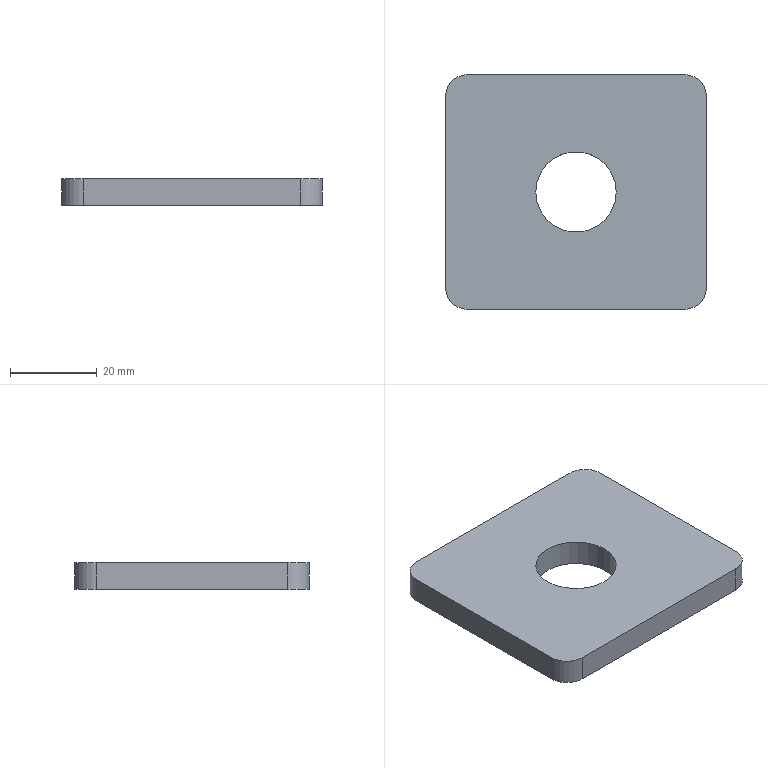Part | STEP file | JBJ-P-1015-03 | 1 solid | 11 faces | box 60 x 54 x 6 mm | volume 17698 mm3 | plane 6 | cylinder 5 | commonest cylinder face diameters 10 x4 18.5 x1
STEP:
#1=CARTESIAN_POINT('',(0.,-5.,0.));
#2=VERTEX_POINT('',#1);
#3=CARTESIAN_POINT('',(0.,-49.,0.));
#4=VERTEX_POINT('',#3);
#5=CARTESIAN_POINT('',(0.,0.,0.));
#6=DIRECTION('',(0.,-1.,0.));
#7=VECTOR('',#6,1000.);
#8=LINE('',#5,#7);
#9=EDGE_CURVE('',#2,#4,#8,.T.);
#10=ORIENTED_EDGE('',*,*,#9,.T.);
#11=CARTESIAN_POINT('',(0.,-49.,6.));
#12=VERTEX_POINT('',#11);
#13=CARTESIAN_POINT('',(0.,-49.,6.));
#14=DIRECTION('',(0.,0.,1.));
#15=VECTOR('',#14,1000.);
#16=LINE('',#13,#15);
#17=EDGE_CURVE('',#4,#12,#16,.T.);
#18=ORIENTED_EDGE('',*,*,#17,.T.);
#19=CARTESIAN_POINT('',(0.,-5.,6.));
#20=VERTEX_POINT('',#19);
#21=CARTESIAN_POINT('',(0.,0.,6.));
#22=DIRECTION('',(0.,-1.,0.));
#23=VECTOR('',#22,1000.);
#24=LINE('',#21,#23);
#25=EDGE_CURVE('',#20,#12,#24,.T.);
#26=ORIENTED_EDGE('',*,*,#25,.F.);
#27=CARTESIAN_POINT('',(0.,-5.,6.));
#28=DIRECTION('',(0.,0.,-1.));
#29=VECTOR('',#28,1000.);
#30=LINE('',#27,#29);
#31=EDGE_CURVE('',#20,#2,#30,.T.);
#32=ORIENTED_EDGE('',*,*,#31,.T.);
#33=EDGE_LOOP('',(#10,#18,#26,#32));
#34=FACE_OUTER_BOUND('',#33,.T.);
#35=CARTESIAN_POINT('',(0.,0.,6.));
#36=DIRECTION('',(1.,0.,0.));
#37=DIRECTION('',(0.,1.,0.));
#38=AXIS2_PLACEMENT_3D('',#35,#36,#37);
#39=PLANE('',#38);
#40=ADVANCED_FACE('',(#34),#39,.F.);
#41=CARTESIAN_POINT('',(5.,-54.,0.));
#42=VERTEX_POINT('',#41);
#43=CARTESIAN_POINT('',(55.,-54.,0.));
#44=VERTEX_POINT('',#43);
#45=CARTESIAN_POINT('',(0.,-54.,0.));
#46=DIRECTION('',(1.,0.,0.));
#47=VECTOR('',#46,1000.);
#48=LINE('',#45,#47);
#49=EDGE_CURVE('',#42,#44,#48,.T.);
#50=ORIENTED_EDGE('',*,*,#49,.T.);
#51=CARTESIAN_POINT('',(55.,-54.,6.));
#52=VERTEX_POINT('',#51);
#53=CARTESIAN_POINT('',(55.,-54.,6.));
#54=DIRECTION('',(0.,0.,1.));
#55=VECTOR('',#54,1000.);
#56=LINE('',#53,#55);
#57=EDGE_CURVE('',#44,#52,#56,.T.);
#58=ORIENTED_EDGE('',*,*,#57,.T.);
#59=CARTESIAN_POINT('',(5.,-54.,6.));
#60=VERTEX_POINT('',#59);
#61=CARTESIAN_POINT('',(0.,-54.,6.));
#62=DIRECTION('',(1.,0.,0.));
#63=VECTOR('',#62,1000.);
#64=LINE('',#61,#63);
#65=EDGE_CURVE('',#60,#52,#64,.T.);
#66=ORIENTED_EDGE('',*,*,#65,.F.);
#67=CARTESIAN_POINT('',(5.,-54.,6.));
#68=DIRECTION('',(0.,0.,-1.));
#69=VECTOR('',#68,1000.);
#70=LINE('',#67,#69);
#71=EDGE_CURVE('',#60,#42,#70,.T.);
#72=ORIENTED_EDGE('',*,*,#71,.T.);
#73=EDGE_LOOP('',(#50,#58,#66,#72));
#74=FACE_OUTER_BOUND('',#73,.T.);
#75=CARTESIAN_POINT('',(0.,-54.,6.));
#76=DIRECTION('',(0.,1.,0.));
#77=DIRECTION('',(0.,0.,1.));
#78=AXIS2_PLACEMENT_3D('',#75,#76,#77);
#79=PLANE('',#78);
#80=ADVANCED_FACE('',(#74),#79,.F.);
#81=CARTESIAN_POINT('',(60.,-49.,0.));
#82=VERTEX_POINT('',#81);
#83=CARTESIAN_POINT('',(60.,-5.,0.));
#84=VERTEX_POINT('',#83);
#85=CARTESIAN_POINT('',(60.,0.,0.));
#86=DIRECTION('',(0.,1.,0.));
#87=VECTOR('',#86,1000.);
#88=LINE('',#85,#87);
#89=EDGE_CURVE('',#82,#84,#88,.T.);
#90=ORIENTED_EDGE('',*,*,#89,.T.);
#91=CARTESIAN_POINT('',(60.,-5.,6.));
#92=VERTEX_POINT('',#91);
#93=CARTESIAN_POINT('',(60.,-5.,6.));
#94=DIRECTION('',(0.,0.,1.));
#95=VECTOR('',#94,1000.);
#96=LINE('',#93,#95);
#97=EDGE_CURVE('',#84,#92,#96,.T.);
#98=ORIENTED_EDGE('',*,*,#97,.T.);
#99=CARTESIAN_POINT('',(60.,-49.,6.));
#100=VERTEX_POINT('',#99);
#101=CARTESIAN_POINT('',(60.,0.,6.));
#102=DIRECTION('',(0.,1.,0.));
#103=VECTOR('',#102,1000.);
#104=LINE('',#101,#103);
#105=EDGE_CURVE('',#100,#92,#104,.T.);
#106=ORIENTED_EDGE('',*,*,#105,.F.);
#107=CARTESIAN_POINT('',(60.,-49.,6.));
#108=DIRECTION('',(0.,0.,-1.));
#109=VECTOR('',#108,1000.);
#110=LINE('',#107,#109);
#111=EDGE_CURVE('',#100,#82,#110,.T.);
#112=ORIENTED_EDGE('',*,*,#111,.T.);
#113=EDGE_LOOP('',(#90,#98,#106,#112));
#114=FACE_OUTER_BOUND('',#113,.T.);
#115=CARTESIAN_POINT('',(60.,0.,6.));
#116=DIRECTION('',(-1.,0.,0.));
#117=DIRECTION('',(0.,-1.,0.));
#118=AXIS2_PLACEMENT_3D('',#115,#116,#117);
#119=PLANE('',#118);
#120=ADVANCED_FACE('',(#114),#119,.F.);
#121=CARTESIAN_POINT('',(55.,0.,6.));
#122=VERTEX_POINT('',#121);
#123=CARTESIAN_POINT('',(5.,0.,6.));
#124=VERTEX_POINT('',#123);
#125=CARTESIAN_POINT('',(0.,0.,6.));
#126=DIRECTION('',(-1.,0.,0.));
#127=VECTOR('',#126,1000.);
#128=LINE('',#125,#127);
#129=EDGE_CURVE('',#122,#124,#128,.T.);
#130=ORIENTED_EDGE('',*,*,#129,.F.);
#131=CARTESIAN_POINT('',(55.,0.,0.));
#132=VERTEX_POINT('',#131);
#133=CARTESIAN_POINT('',(55.,0.,6.));
#134=DIRECTION('',(0.,0.,-1.));
#135=VECTOR('',#134,1000.);
#136=LINE('',#133,#135);
#137=EDGE_CURVE('',#122,#132,#136,.T.);
#138=ORIENTED_EDGE('',*,*,#137,.T.);
#139=CARTESIAN_POINT('',(5.,0.,0.));
#140=VERTEX_POINT('',#139);
#141=CARTESIAN_POINT('',(0.,0.,0.));
#142=DIRECTION('',(-1.,0.,0.));
#143=VECTOR('',#142,1000.);
#144=LINE('',#141,#143);
#145=EDGE_CURVE('',#132,#140,#144,.T.);
#146=ORIENTED_EDGE('',*,*,#145,.T.);
#147=CARTESIAN_POINT('',(5.,0.,6.));
#148=DIRECTION('',(0.,0.,1.));
#149=VECTOR('',#148,1000.);
#150=LINE('',#147,#149);
#151=EDGE_CURVE('',#140,#124,#150,.T.);
#152=ORIENTED_EDGE('',*,*,#151,.T.);
#153=EDGE_LOOP('',(#130,#138,#146,#152));
#154=FACE_OUTER_BOUND('',#153,.T.);
#155=CARTESIAN_POINT('',(0.,0.,6.));
#156=DIRECTION('',(0.,-1.,0.));
#157=DIRECTION('',(0.,0.,-1.));
#158=AXIS2_PLACEMENT_3D('',#155,#156,#157);
#159=PLANE('',#158);
#160=ADVANCED_FACE('',(#154),#159,.F.);
#161=CARTESIAN_POINT('',(39.25,-27.,6.));
#162=VERTEX_POINT('',#161);
#163=CARTESIAN_POINT('',(30.,-27.,6.));
#164=DIRECTION('',(0.,0.,1.));
#165=DIRECTION('',(1.,0.,0.));
#166=AXIS2_PLACEMENT_3D('',#163,#164,#165);
#167=CIRCLE('',#166,9.25);
#168=EDGE_CURVE('',#162,#162,#167,.T.);
#169=ORIENTED_EDGE('',*,*,#168,.F.);
#170=EDGE_LOOP('',(#169));
#171=FACE_BOUND('',#170,.T.);
#172=ORIENTED_EDGE('',*,*,#105,.T.);
#173=CARTESIAN_POINT('',(55.,-5.,6.));
#174=DIRECTION('',(0.,0.,1.));
#175=DIRECTION('',(1.,0.,0.));
#176=AXIS2_PLACEMENT_3D('',#173,#174,#175);
#177=CIRCLE('',#176,5.);
#178=EDGE_CURVE('',#92,#122,#177,.T.);
#179=ORIENTED_EDGE('',*,*,#178,.T.);
#180=ORIENTED_EDGE('',*,*,#129,.T.);
#181=CARTESIAN_POINT('',(5.,-5.,6.));
#182=DIRECTION('',(0.,0.,1.));
#183=DIRECTION('',(1.,0.,0.));
#184=AXIS2_PLACEMENT_3D('',#181,#182,#183);
#185=CIRCLE('',#184,5.);
#186=EDGE_CURVE('',#124,#20,#185,.T.);
#187=ORIENTED_EDGE('',*,*,#186,.T.);
#188=ORIENTED_EDGE('',*,*,#25,.T.);
#189=CARTESIAN_POINT('',(5.,-49.,6.));
#190=DIRECTION('',(0.,0.,1.));
#191=DIRECTION('',(1.,0.,0.));
#192=AXIS2_PLACEMENT_3D('',#189,#190,#191);
#193=CIRCLE('',#192,5.);
#194=EDGE_CURVE('',#12,#60,#193,.T.);
#195=ORIENTED_EDGE('',*,*,#194,.T.);
#196=ORIENTED_EDGE('',*,*,#65,.T.);
#197=CARTESIAN_POINT('',(55.,-49.,6.));
#198=DIRECTION('',(0.,0.,1.));
#199=DIRECTION('',(1.,0.,0.));
#200=AXIS2_PLACEMENT_3D('',#197,#198,#199);
#201=CIRCLE('',#200,5.);
#202=EDGE_CURVE('',#52,#100,#201,.T.);
#203=ORIENTED_EDGE('',*,*,#202,.T.);
#204=EDGE_LOOP('',(#172,#179,#180,#187,#188,#195,#196,#203));
#205=FACE_OUTER_BOUND('',#204,.T.);
#206=CARTESIAN_POINT('',(0.,0.,6.));
#207=DIRECTION('',(0.,0.,1.));
#208=DIRECTION('',(1.,0.,0.));
#209=AXIS2_PLACEMENT_3D('',#206,#207,#208);
#210=PLANE('',#209);
#211=ADVANCED_FACE('',(#171,#205),#210,.T.);
#212=CARTESIAN_POINT('',(39.25,-27.,0.));
#213=VERTEX_POINT('',#212);
#214=CARTESIAN_POINT('',(30.,-27.,0.));
#215=DIRECTION('',(0.,0.,1.));
#216=DIRECTION('',(1.,0.,0.));
#217=AXIS2_PLACEMENT_3D('',#214,#215,#216);
#218=CIRCLE('',#217,9.25);
#219=EDGE_CURVE('',#213,#213,#218,.T.);
#220=ORIENTED_EDGE('',*,*,#219,.T.);
#221=EDGE_LOOP('',(#220));
#222=FACE_BOUND('',#221,.T.);
#223=ORIENTED_EDGE('',*,*,#145,.F.);
#224=CARTESIAN_POINT('',(55.,-5.,0.));
#225=DIRECTION('',(0.,0.,-1.));
#226=DIRECTION('',(1.,0.,0.));
#227=AXIS2_PLACEMENT_3D('',#224,#225,#226);
#228=CIRCLE('',#227,5.);
#229=EDGE_CURVE('',#132,#84,#228,.T.);
#230=ORIENTED_EDGE('',*,*,#229,.T.);
#231=ORIENTED_EDGE('',*,*,#89,.F.);
#232=CARTESIAN_POINT('',(55.,-49.,0.));
#233=DIRECTION('',(0.,0.,-1.));
#234=DIRECTION('',(1.,0.,0.));
#235=AXIS2_PLACEMENT_3D('',#232,#233,#234);
#236=CIRCLE('',#235,5.);
#237=EDGE_CURVE('',#82,#44,#236,.T.);
#238=ORIENTED_EDGE('',*,*,#237,.T.);
#239=ORIENTED_EDGE('',*,*,#49,.F.);
#240=CARTESIAN_POINT('',(5.,-49.,0.));
#241=DIRECTION('',(0.,0.,-1.));
#242=DIRECTION('',(1.,0.,0.));
#243=AXIS2_PLACEMENT_3D('',#240,#241,#242);
#244=CIRCLE('',#243,5.);
#245=EDGE_CURVE('',#42,#4,#244,.T.);
#246=ORIENTED_EDGE('',*,*,#245,.T.);
#247=ORIENTED_EDGE('',*,*,#9,.F.);
#248=CARTESIAN_POINT('',(5.,-5.,0.));
#249=DIRECTION('',(0.,0.,-1.));
#250=DIRECTION('',(1.,0.,0.));
#251=AXIS2_PLACEMENT_3D('',#248,#249,#250);
#252=CIRCLE('',#251,5.);
#253=EDGE_CURVE('',#2,#140,#252,.T.);
#254=ORIENTED_EDGE('',*,*,#253,.T.);
#255=EDGE_LOOP('',(#223,#230,#231,#238,#239,#246,#247,#254));
#256=FACE_OUTER_BOUND('',#255,.T.);
#257=CARTESIAN_POINT('',(0.,0.,0.));
#258=DIRECTION('',(0.,0.,1.));
#259=DIRECTION('',(1.,0.,0.));
#260=AXIS2_PLACEMENT_3D('',#257,#258,#259);
#261=PLANE('',#260);
#262=ADVANCED_FACE('',(#222,#256),#261,.F.);
#263=ORIENTED_EDGE('',*,*,#219,.F.);
#264=EDGE_LOOP('',(#263));
#265=FACE_OUTER_BOUND('',#264,.T.);
#266=ORIENTED_EDGE('',*,*,#168,.T.);
#267=EDGE_LOOP('',(#266));
#268=FACE_OUTER_BOUND('',#267,.T.);
#269=CARTESIAN_POINT('',(30.,-27.,6.));
#270=DIRECTION('',(0.,0.,1.));
#271=DIRECTION('',(1.,0.,0.));
#272=AXIS2_PLACEMENT_3D('',#269,#270,#271);
#273=CYLINDRICAL_SURFACE('',#272,9.25);
#274=ADVANCED_FACE('',(#265,#268),#273,.F.);
#275=ORIENTED_EDGE('',*,*,#178,.F.);
#276=ORIENTED_EDGE('',*,*,#97,.F.);
#277=ORIENTED_EDGE('',*,*,#229,.F.);
#278=ORIENTED_EDGE('',*,*,#137,.F.);
#279=EDGE_LOOP('',(#275,#276,#277,#278));
#280=FACE_OUTER_BOUND('',#279,.T.);
#281=CARTESIAN_POINT('',(55.,-5.,6.));
#282=DIRECTION('',(0.,0.,-1.));
#283=DIRECTION('',(-1.,0.,0.));
#284=AXIS2_PLACEMENT_3D('',#281,#282,#283);
#285=CYLINDRICAL_SURFACE('',#284,5.);
#286=ADVANCED_FACE('',(#280),#285,.T.);
#287=ORIENTED_EDGE('',*,*,#202,.F.);
#288=ORIENTED_EDGE('',*,*,#57,.F.);
#289=ORIENTED_EDGE('',*,*,#237,.F.);
#290=ORIENTED_EDGE('',*,*,#111,.F.);
#291=EDGE_LOOP('',(#287,#288,#289,#290));
#292=FACE_OUTER_BOUND('',#291,.T.);
#293=CARTESIAN_POINT('',(55.,-49.,6.));
#294=DIRECTION('',(0.,0.,-1.));
#295=DIRECTION('',(-1.,0.,0.));
#296=AXIS2_PLACEMENT_3D('',#293,#294,#295);
#297=CYLINDRICAL_SURFACE('',#296,5.);
#298=ADVANCED_FACE('',(#292),#297,.T.);
#299=ORIENTED_EDGE('',*,*,#194,.F.);
#300=ORIENTED_EDGE('',*,*,#17,.F.);
#301=ORIENTED_EDGE('',*,*,#245,.F.);
#302=ORIENTED_EDGE('',*,*,#71,.F.);
#303=EDGE_LOOP('',(#299,#300,#301,#302));
#304=FACE_OUTER_BOUND('',#303,.T.);
#305=CARTESIAN_POINT('',(5.,-49.,6.));
#306=DIRECTION('',(0.,0.,-1.));
#307=DIRECTION('',(-1.,0.,0.));
#308=AXIS2_PLACEMENT_3D('',#305,#306,#307);
#309=CYLINDRICAL_SURFACE('',#308,5.);
#310=ADVANCED_FACE('',(#304),#309,.T.);
#311=ORIENTED_EDGE('',*,*,#186,.F.);
#312=ORIENTED_EDGE('',*,*,#151,.F.);
#313=ORIENTED_EDGE('',*,*,#253,.F.);
#314=ORIENTED_EDGE('',*,*,#31,.F.);
#315=EDGE_LOOP('',(#311,#312,#313,#314));
#316=FACE_OUTER_BOUND('',#315,.T.);
#317=CARTESIAN_POINT('',(5.,-5.,6.));
#318=DIRECTION('',(0.,0.,-1.));
#319=DIRECTION('',(-1.,0.,0.));
#320=AXIS2_PLACEMENT_3D('',#317,#318,#319);
#321=CYLINDRICAL_SURFACE('',#320,5.);
#322=ADVANCED_FACE('',(#316),#321,.T.);
#323=CLOSED_SHELL('',(#40,#80,#120,#160,#211,#262,#274,#286,#298,#310,#322));
#324=MANIFOLD_SOLID_BREP('',#323);
#325=CARTESIAN_POINT('',(0.,0.,0.));
#326=DIRECTION('',(0.,0.,1.));
#327=DIRECTION('',(1.,0.,0.));
#328=AXIS2_PLACEMENT_3D('',#325,#326,#327);
#329=(LENGTH_UNIT()NAMED_UNIT(*)SI_UNIT(.MILLI.,.METRE.));
#330=UNCERTAINTY_MEASURE_WITH_UNIT(LENGTH_MEASURE(0.00001),#329,'','');
#331=(NAMED_UNIT(*)PLANE_ANGLE_UNIT()SI_UNIT($,.RADIAN.));
#332=(NAMED_UNIT(*)SI_UNIT($,.STERADIAN.)SOLID_ANGLE_UNIT());
#333=(GEOMETRIC_REPRESENTATION_CONTEXT(3)GLOBAL_UNCERTAINTY_ASSIGNED_CONTEXT((#330))GLOBAL_UNIT_ASSIGNED_CONTEXT((#329,#331,#332))REPRESENTATION_CONTEXT('',''));
#334=ADVANCED_BREP_SHAPE_REPRESENTATION('',(#324,#328),#333);